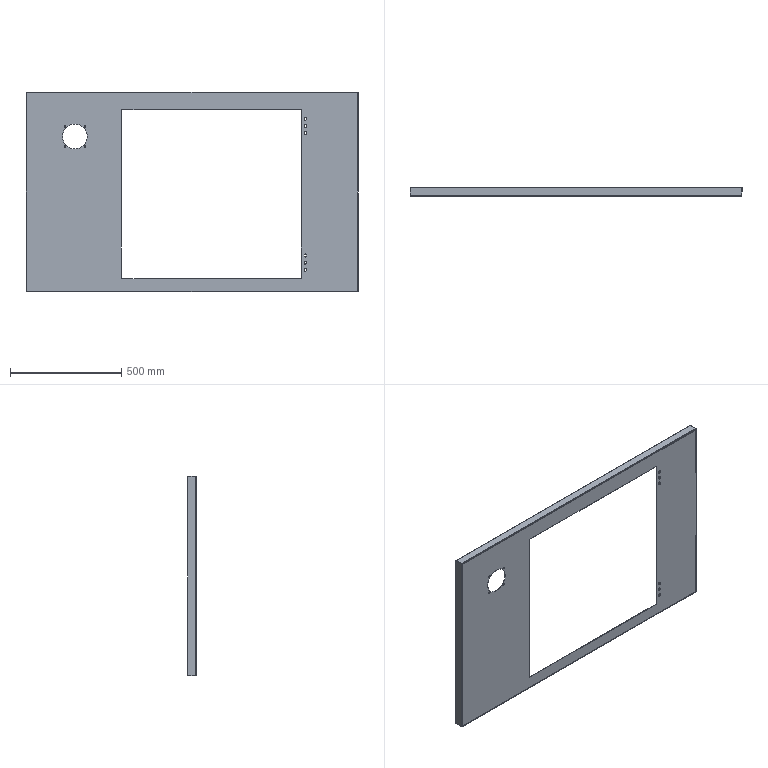Part | SolidWorks | features ICE 3, EdgeFlange 1, FlatPattern 1, SMBaseFlange 1, SheetMetal 1 | 1 solid | 86 faces | box 1495 x 40 x 900 mm | volume 1788813 mm3 | cylinder 40 | plane 38 | spline 8 | commonest cylinder face diameters 9 x18 4 x8 7.5 x8 8 x4 112 x2